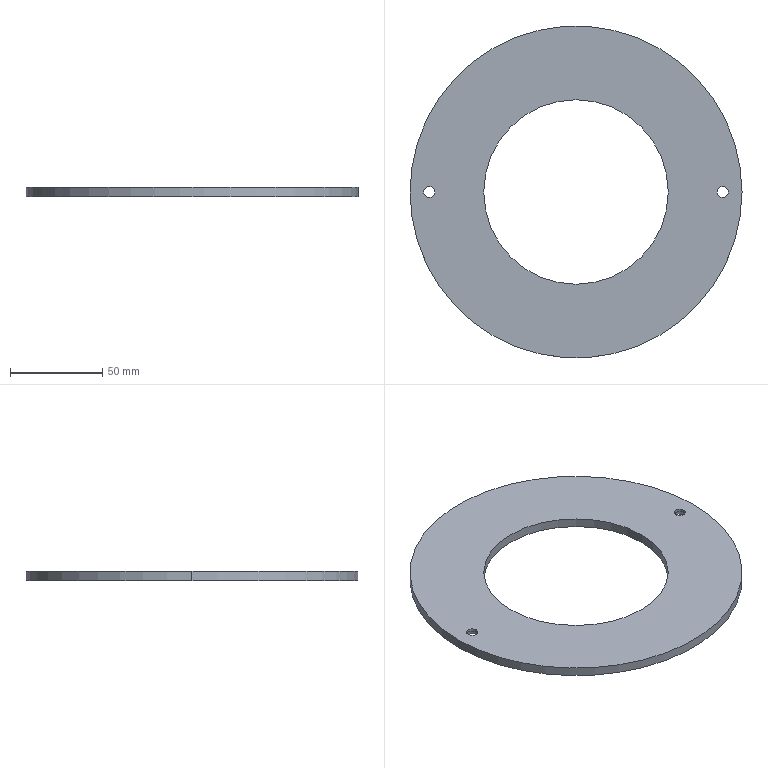Part | STEP file | Spacer block | 1 solid | 16 faces | box 180 x 180 x 5 mm | volume 87215 mm3 | cylinder 12 | plane 4 | commonest cylinder face diameters 6 x4 11 x4 100 x2 180 x2
STEP:
#1=CARTESIAN_POINT('',(85.05,0.,3.5));
#2=VERTEX_POINT('',#1);
#3=CARTESIAN_POINT('',(74.05,0.,3.5));
#4=VERTEX_POINT('',#3);
#5=CARTESIAN_POINT('',(79.55,0.,3.5));
#6=DIRECTION('',(0.,0.,-1.));
#7=DIRECTION('',(-1.,0.,0.));
#8=AXIS2_PLACEMENT_3D('',#5,#6,#7);
#9=CIRCLE('',#8,5.5);
#10=EDGE_CURVE('',#2,#4,#9,.T.);
#11=ORIENTED_EDGE('',*,*,#10,.F.);
#12=CARTESIAN_POINT('',(85.05,0.,0.));
#13=VERTEX_POINT('',#12);
#14=CARTESIAN_POINT('',(85.05,0.,3.5));
#15=DIRECTION('',(0.,0.,-1.));
#16=VECTOR('',#15,1000.);
#17=LINE('',#14,#16);
#18=EDGE_CURVE('',#2,#13,#17,.T.);
#19=ORIENTED_EDGE('',*,*,#18,.T.);
#20=CARTESIAN_POINT('',(74.05,0.,0.));
#21=VERTEX_POINT('',#20);
#22=CARTESIAN_POINT('',(79.55,0.,0.));
#23=DIRECTION('',(0.,0.,-1.));
#24=DIRECTION('',(-1.,0.,0.));
#25=AXIS2_PLACEMENT_3D('',#22,#23,#24);
#26=CIRCLE('',#25,5.5);
#27=EDGE_CURVE('',#13,#21,#26,.T.);
#28=ORIENTED_EDGE('',*,*,#27,.T.);
#29=CARTESIAN_POINT('',(74.05,0.,3.5));
#30=DIRECTION('',(0.,0.,-1.));
#31=VECTOR('',#30,1000.);
#32=LINE('',#29,#31);
#33=EDGE_CURVE('',#4,#21,#32,.T.);
#34=ORIENTED_EDGE('',*,*,#33,.F.);
#35=EDGE_LOOP('',(#11,#19,#28,#34));
#36=FACE_OUTER_BOUND('',#35,.T.);
#37=CARTESIAN_POINT('',(79.55,0.,3.5));
#38=DIRECTION('',(0.,0.,-1.));
#39=DIRECTION('',(-1.,0.,0.));
#40=AXIS2_PLACEMENT_3D('',#37,#38,#39);
#41=CYLINDRICAL_SURFACE('',#40,5.5);
#42=ADVANCED_FACE('',(#36),#41,.F.);
#43=CARTESIAN_POINT('',(-74.05,0.,3.5));
#44=VERTEX_POINT('',#43);
#45=CARTESIAN_POINT('',(-85.05,0.,3.5));
#46=VERTEX_POINT('',#45);
#47=CARTESIAN_POINT('',(-79.55,0.,3.5));
#48=DIRECTION('',(0.,0.,-1.));
#49=DIRECTION('',(-1.,0.,0.));
#50=AXIS2_PLACEMENT_3D('',#47,#48,#49);
#51=CIRCLE('',#50,5.5);
#52=EDGE_CURVE('',#44,#46,#51,.T.);
#53=ORIENTED_EDGE('',*,*,#52,.F.);
#54=CARTESIAN_POINT('',(-74.05,0.,0.));
#55=VERTEX_POINT('',#54);
#56=CARTESIAN_POINT('',(-74.05,0.,3.5));
#57=DIRECTION('',(0.,0.,-1.));
#58=VECTOR('',#57,1000.);
#59=LINE('',#56,#58);
#60=EDGE_CURVE('',#44,#55,#59,.T.);
#61=ORIENTED_EDGE('',*,*,#60,.T.);
#62=CARTESIAN_POINT('',(-85.05,0.,0.));
#63=VERTEX_POINT('',#62);
#64=CARTESIAN_POINT('',(-79.55,0.,0.));
#65=DIRECTION('',(0.,0.,-1.));
#66=DIRECTION('',(-1.,0.,0.));
#67=AXIS2_PLACEMENT_3D('',#64,#65,#66);
#68=CIRCLE('',#67,5.5);
#69=EDGE_CURVE('',#55,#63,#68,.T.);
#70=ORIENTED_EDGE('',*,*,#69,.T.);
#71=CARTESIAN_POINT('',(-85.05,0.,3.5));
#72=DIRECTION('',(0.,0.,-1.));
#73=VECTOR('',#72,1000.);
#74=LINE('',#71,#73);
#75=EDGE_CURVE('',#46,#63,#74,.T.);
#76=ORIENTED_EDGE('',*,*,#75,.F.);
#77=EDGE_LOOP('',(#53,#61,#70,#76));
#78=FACE_OUTER_BOUND('',#77,.T.);
#79=CARTESIAN_POINT('',(-79.55,0.,3.5));
#80=DIRECTION('',(0.,0.,-1.));
#81=DIRECTION('',(-1.,0.,0.));
#82=AXIS2_PLACEMENT_3D('',#79,#80,#81);
#83=CYLINDRICAL_SURFACE('',#82,5.5);
#84=ADVANCED_FACE('',(#78),#83,.F.);
#85=CARTESIAN_POINT('',(-50.,0.,5.));
#86=VERTEX_POINT('',#85);
#87=CARTESIAN_POINT('',(50.,0.,5.));
#88=VERTEX_POINT('',#87);
#89=CARTESIAN_POINT('',(0.,0.,5.));
#90=DIRECTION('',(0.,0.,1.));
#91=DIRECTION('',(1.,0.,0.));
#92=AXIS2_PLACEMENT_3D('',#89,#90,#91);
#93=CIRCLE('',#92,50.);
#94=EDGE_CURVE('',#86,#88,#93,.T.);
#95=ORIENTED_EDGE('',*,*,#94,.T.);
#96=CARTESIAN_POINT('',(50.,0.,0.));
#97=VERTEX_POINT('',#96);
#98=CARTESIAN_POINT('',(50.,0.,5.));
#99=DIRECTION('',(0.,0.,-1.));
#100=VECTOR('',#99,1000.);
#101=LINE('',#98,#100);
#102=EDGE_CURVE('',#88,#97,#101,.T.);
#103=ORIENTED_EDGE('',*,*,#102,.T.);
#104=CARTESIAN_POINT('',(-50.,0.,0.));
#105=VERTEX_POINT('',#104);
#106=CARTESIAN_POINT('',(0.,0.,0.));
#107=DIRECTION('',(0.,0.,1.));
#108=DIRECTION('',(1.,0.,0.));
#109=AXIS2_PLACEMENT_3D('',#106,#107,#108);
#110=CIRCLE('',#109,50.);
#111=EDGE_CURVE('',#105,#97,#110,.T.);
#112=ORIENTED_EDGE('',*,*,#111,.F.);
#113=CARTESIAN_POINT('',(-50.,0.,5.));
#114=DIRECTION('',(0.,0.,-1.));
#115=VECTOR('',#114,1000.);
#116=LINE('',#113,#115);
#117=EDGE_CURVE('',#86,#105,#116,.T.);
#118=ORIENTED_EDGE('',*,*,#117,.F.);
#119=EDGE_LOOP('',(#95,#103,#112,#118));
#120=FACE_OUTER_BOUND('',#119,.T.);
#121=CARTESIAN_POINT('',(0.,0.,5.));
#122=DIRECTION('',(0.,0.,-1.));
#123=DIRECTION('',(-1.,0.,0.));
#124=AXIS2_PLACEMENT_3D('',#121,#122,#123);
#125=CYLINDRICAL_SURFACE('',#124,50.);
#126=ADVANCED_FACE('',(#120),#125,.F.);
#127=CARTESIAN_POINT('',(90.,0.,5.));
#128=VERTEX_POINT('',#127);
#129=CARTESIAN_POINT('',(-90.,0.,5.));
#130=VERTEX_POINT('',#129);
#131=CARTESIAN_POINT('',(0.,0.,5.));
#132=DIRECTION('',(0.,0.,1.));
#133=DIRECTION('',(1.,0.,0.));
#134=AXIS2_PLACEMENT_3D('',#131,#132,#133);
#135=CIRCLE('',#134,90.);
#136=EDGE_CURVE('',#128,#130,#135,.T.);
#137=ORIENTED_EDGE('',*,*,#136,.F.);
#138=CARTESIAN_POINT('',(90.,0.,0.));
#139=VERTEX_POINT('',#138);
#140=CARTESIAN_POINT('',(90.,0.,5.));
#141=DIRECTION('',(0.,0.,-1.));
#142=VECTOR('',#141,1000.);
#143=LINE('',#140,#142);
#144=EDGE_CURVE('',#128,#139,#143,.T.);
#145=ORIENTED_EDGE('',*,*,#144,.T.);
#146=CARTESIAN_POINT('',(-90.,0.,0.));
#147=VERTEX_POINT('',#146);
#148=CARTESIAN_POINT('',(0.,0.,0.));
#149=DIRECTION('',(0.,0.,1.));
#150=DIRECTION('',(1.,0.,0.));
#151=AXIS2_PLACEMENT_3D('',#148,#149,#150);
#152=CIRCLE('',#151,90.);
#153=EDGE_CURVE('',#139,#147,#152,.T.);
#154=ORIENTED_EDGE('',*,*,#153,.T.);
#155=CARTESIAN_POINT('',(-90.,0.,5.));
#156=DIRECTION('',(0.,0.,-1.));
#157=VECTOR('',#156,1000.);
#158=LINE('',#155,#157);
#159=EDGE_CURVE('',#130,#147,#158,.T.);
#160=ORIENTED_EDGE('',*,*,#159,.F.);
#161=EDGE_LOOP('',(#137,#145,#154,#160));
#162=FACE_OUTER_BOUND('',#161,.T.);
#163=CARTESIAN_POINT('',(0.,0.,5.));
#164=DIRECTION('',(0.,0.,-1.));
#165=DIRECTION('',(-1.,0.,0.));
#166=AXIS2_PLACEMENT_3D('',#163,#164,#165);
#167=CYLINDRICAL_SURFACE('',#166,90.);
#168=ADVANCED_FACE('',(#162),#167,.T.);
#169=CARTESIAN_POINT('',(-82.55,0.,3.5));
#170=VERTEX_POINT('',#169);
#171=CARTESIAN_POINT('',(-76.55,0.,3.5));
#172=VERTEX_POINT('',#171);
#173=CARTESIAN_POINT('',(-79.55,0.,3.5));
#174=DIRECTION('',(0.,0.,1.));
#175=DIRECTION('',(-1.,0.,0.));
#176=AXIS2_PLACEMENT_3D('',#173,#174,#175);
#177=CIRCLE('',#176,3.);
#178=EDGE_CURVE('',#170,#172,#177,.T.);
#179=ORIENTED_EDGE('',*,*,#178,.F.);
#180=CARTESIAN_POINT('',(-82.55,0.,5.));
#181=VERTEX_POINT('',#180);
#182=CARTESIAN_POINT('',(-82.55,0.,-5.));
#183=DIRECTION('',(0.,0.,1.));
#184=VECTOR('',#183,1000.);
#185=LINE('',#182,#184);
#186=EDGE_CURVE('',#170,#181,#185,.T.);
#187=ORIENTED_EDGE('',*,*,#186,.T.);
#188=CARTESIAN_POINT('',(-76.55,0.,5.));
#189=VERTEX_POINT('',#188);
#190=CARTESIAN_POINT('',(-79.55,0.,5.));
#191=DIRECTION('',(0.,0.,1.));
#192=DIRECTION('',(1.,0.,0.));
#193=AXIS2_PLACEMENT_3D('',#190,#191,#192);
#194=CIRCLE('',#193,3.);
#195=EDGE_CURVE('',#181,#189,#194,.T.);
#196=ORIENTED_EDGE('',*,*,#195,.T.);
#197=CARTESIAN_POINT('',(-76.55,0.,-5.));
#198=DIRECTION('',(0.,0.,1.));
#199=VECTOR('',#198,1000.);
#200=LINE('',#197,#199);
#201=EDGE_CURVE('',#172,#189,#200,.T.);
#202=ORIENTED_EDGE('',*,*,#201,.F.);
#203=EDGE_LOOP('',(#179,#187,#196,#202));
#204=FACE_OUTER_BOUND('',#203,.T.);
#205=CARTESIAN_POINT('',(-79.55,0.,-5.));
#206=DIRECTION('',(0.,0.,1.));
#207=DIRECTION('',(1.,0.,0.));
#208=AXIS2_PLACEMENT_3D('',#205,#206,#207);
#209=CYLINDRICAL_SURFACE('',#208,3.);
#210=ADVANCED_FACE('',(#204),#209,.F.);
#211=CARTESIAN_POINT('',(76.55,0.,3.5));
#212=VERTEX_POINT('',#211);
#213=CARTESIAN_POINT('',(82.55,0.,3.5));
#214=VERTEX_POINT('',#213);
#215=CARTESIAN_POINT('',(79.55,0.,3.5));
#216=DIRECTION('',(0.,0.,1.));
#217=DIRECTION('',(-1.,0.,0.));
#218=AXIS2_PLACEMENT_3D('',#215,#216,#217);
#219=CIRCLE('',#218,3.);
#220=EDGE_CURVE('',#212,#214,#219,.T.);
#221=ORIENTED_EDGE('',*,*,#220,.F.);
#222=CARTESIAN_POINT('',(76.55,0.,5.));
#223=VERTEX_POINT('',#222);
#224=CARTESIAN_POINT('',(76.55,0.,-5.));
#225=DIRECTION('',(0.,0.,1.));
#226=VECTOR('',#225,1000.);
#227=LINE('',#224,#226);
#228=EDGE_CURVE('',#212,#223,#227,.T.);
#229=ORIENTED_EDGE('',*,*,#228,.T.);
#230=CARTESIAN_POINT('',(82.55,0.,5.));
#231=VERTEX_POINT('',#230);
#232=CARTESIAN_POINT('',(79.55,0.,5.));
#233=DIRECTION('',(0.,0.,1.));
#234=DIRECTION('',(1.,0.,0.));
#235=AXIS2_PLACEMENT_3D('',#232,#233,#234);
#236=CIRCLE('',#235,3.);
#237=EDGE_CURVE('',#223,#231,#236,.T.);
#238=ORIENTED_EDGE('',*,*,#237,.T.);
#239=CARTESIAN_POINT('',(82.55,0.,-5.));
#240=DIRECTION('',(0.,0.,1.));
#241=VECTOR('',#240,1000.);
#242=LINE('',#239,#241);
#243=EDGE_CURVE('',#214,#231,#242,.T.);
#244=ORIENTED_EDGE('',*,*,#243,.F.);
#245=EDGE_LOOP('',(#221,#229,#238,#244));
#246=FACE_OUTER_BOUND('',#245,.T.);
#247=CARTESIAN_POINT('',(79.55,0.,-5.));
#248=DIRECTION('',(0.,0.,1.));
#249=DIRECTION('',(1.,0.,0.));
#250=AXIS2_PLACEMENT_3D('',#247,#248,#249);
#251=CYLINDRICAL_SURFACE('',#250,3.);
#252=ADVANCED_FACE('',(#246),#251,.F.);
#253=ORIENTED_EDGE('',*,*,#228,.F.);
#254=CARTESIAN_POINT('',(79.55,0.,3.5));
#255=DIRECTION('',(0.,0.,1.));
#256=DIRECTION('',(-1.,0.,0.));
#257=AXIS2_PLACEMENT_3D('',#254,#255,#256);
#258=CIRCLE('',#257,3.);
#259=EDGE_CURVE('',#214,#212,#258,.T.);
#260=ORIENTED_EDGE('',*,*,#259,.F.);
#261=ORIENTED_EDGE('',*,*,#243,.T.);
#262=CARTESIAN_POINT('',(79.55,0.,5.));
#263=DIRECTION('',(0.,0.,1.));
#264=DIRECTION('',(1.,0.,0.));
#265=AXIS2_PLACEMENT_3D('',#262,#263,#264);
#266=CIRCLE('',#265,3.);
#267=EDGE_CURVE('',#231,#223,#266,.T.);
#268=ORIENTED_EDGE('',*,*,#267,.T.);
#269=EDGE_LOOP('',(#253,#260,#261,#268));
#270=FACE_OUTER_BOUND('',#269,.T.);
#271=CARTESIAN_POINT('',(79.55,0.,-5.));
#272=DIRECTION('',(0.,0.,1.));
#273=DIRECTION('',(1.,0.,0.));
#274=AXIS2_PLACEMENT_3D('',#271,#272,#273);
#275=CYLINDRICAL_SURFACE('',#274,3.);
#276=ADVANCED_FACE('',(#270),#275,.F.);
#277=ORIENTED_EDGE('',*,*,#186,.F.);
#278=CARTESIAN_POINT('',(-79.55,0.,3.5));
#279=DIRECTION('',(0.,0.,1.));
#280=DIRECTION('',(-1.,0.,0.));
#281=AXIS2_PLACEMENT_3D('',#278,#279,#280);
#282=CIRCLE('',#281,3.);
#283=EDGE_CURVE('',#172,#170,#282,.T.);
#284=ORIENTED_EDGE('',*,*,#283,.F.);
#285=ORIENTED_EDGE('',*,*,#201,.T.);
#286=CARTESIAN_POINT('',(-79.55,0.,5.));
#287=DIRECTION('',(0.,0.,1.));
#288=DIRECTION('',(1.,0.,0.));
#289=AXIS2_PLACEMENT_3D('',#286,#287,#288);
#290=CIRCLE('',#289,3.);
#291=EDGE_CURVE('',#189,#181,#290,.T.);
#292=ORIENTED_EDGE('',*,*,#291,.T.);
#293=EDGE_LOOP('',(#277,#284,#285,#292));
#294=FACE_OUTER_BOUND('',#293,.T.);
#295=CARTESIAN_POINT('',(-79.55,0.,-5.));
#296=DIRECTION('',(0.,0.,1.));
#297=DIRECTION('',(1.,0.,0.));
#298=AXIS2_PLACEMENT_3D('',#295,#296,#297);
#299=CYLINDRICAL_SURFACE('',#298,3.);
#300=ADVANCED_FACE('',(#294),#299,.F.);
#301=ORIENTED_EDGE('',*,*,#291,.F.);
#302=ORIENTED_EDGE('',*,*,#195,.F.);
#303=EDGE_LOOP('',(#301,#302));
#304=FACE_BOUND('',#303,.T.);
#305=ORIENTED_EDGE('',*,*,#267,.F.);
#306=ORIENTED_EDGE('',*,*,#237,.F.);
#307=EDGE_LOOP('',(#305,#306));
#308=FACE_BOUND('',#307,.T.);
#309=CARTESIAN_POINT('',(0.,0.,5.));
#310=DIRECTION('',(0.,0.,1.));
#311=DIRECTION('',(1.,0.,0.));
#312=AXIS2_PLACEMENT_3D('',#309,#310,#311);
#313=CIRCLE('',#312,90.);
#314=EDGE_CURVE('',#130,#128,#313,.T.);
#315=ORIENTED_EDGE('',*,*,#314,.T.);
#316=ORIENTED_EDGE('',*,*,#136,.T.);
#317=EDGE_LOOP('',(#315,#316));
#318=FACE_OUTER_BOUND('',#317,.T.);
#319=ORIENTED_EDGE('',*,*,#94,.F.);
#320=CARTESIAN_POINT('',(0.,0.,5.));
#321=DIRECTION('',(0.,0.,1.));
#322=DIRECTION('',(1.,0.,0.));
#323=AXIS2_PLACEMENT_3D('',#320,#321,#322);
#324=CIRCLE('',#323,50.);
#325=EDGE_CURVE('',#88,#86,#324,.T.);
#326=ORIENTED_EDGE('',*,*,#325,.F.);
#327=EDGE_LOOP('',(#319,#326));
#328=FACE_BOUND('',#327,.T.);
#329=CARTESIAN_POINT('',(0.,0.,5.));
#330=DIRECTION('',(0.,0.,1.));
#331=DIRECTION('',(1.,0.,0.));
#332=AXIS2_PLACEMENT_3D('',#329,#330,#331);
#333=PLANE('',#332);
#334=ADVANCED_FACE('',(#304,#308,#318,#328),#333,.T.);
#335=CARTESIAN_POINT('',(79.55,0.,0.));
#336=DIRECTION('',(0.,0.,-1.));
#337=DIRECTION('',(-1.,0.,0.));
#338=AXIS2_PLACEMENT_3D('',#335,#336,#337);
#339=CIRCLE('',#338,5.5);
#340=EDGE_CURVE('',#21,#13,#339,.T.);
#341=ORIENTED_EDGE('',*,*,#340,.F.);
#342=ORIENTED_EDGE('',*,*,#27,.F.);
#343=EDGE_LOOP('',(#341,#342));
#344=FACE_BOUND('',#343,.T.);
#345=CARTESIAN_POINT('',(-79.55,0.,0.));
#346=DIRECTION('',(0.,0.,-1.));
#347=DIRECTION('',(-1.,0.,0.));
#348=AXIS2_PLACEMENT_3D('',#345,#346,#347);
#349=CIRCLE('',#348,5.5);
#350=EDGE_CURVE('',#63,#55,#349,.T.);
#351=ORIENTED_EDGE('',*,*,#350,.F.);
#352=ORIENTED_EDGE('',*,*,#69,.F.);
#353=EDGE_LOOP('',(#351,#352));
#354=FACE_BOUND('',#353,.T.);
#355=CARTESIAN_POINT('',(0.,0.,0.));
#356=DIRECTION('',(0.,0.,1.));
#357=DIRECTION('',(1.,0.,0.));
#358=AXIS2_PLACEMENT_3D('',#355,#356,#357);
#359=CIRCLE('',#358,90.);
#360=EDGE_CURVE('',#147,#139,#359,.T.);
#361=ORIENTED_EDGE('',*,*,#360,.F.);
#362=ORIENTED_EDGE('',*,*,#153,.F.);
#363=EDGE_LOOP('',(#361,#362));
#364=FACE_OUTER_BOUND('',#363,.T.);
#365=ORIENTED_EDGE('',*,*,#111,.T.);
#366=CARTESIAN_POINT('',(0.,0.,0.));
#367=DIRECTION('',(0.,0.,1.));
#368=DIRECTION('',(1.,0.,0.));
#369=AXIS2_PLACEMENT_3D('',#366,#367,#368);
#370=CIRCLE('',#369,50.);
#371=EDGE_CURVE('',#97,#105,#370,.T.);
#372=ORIENTED_EDGE('',*,*,#371,.T.);
#373=EDGE_LOOP('',(#365,#372));
#374=FACE_BOUND('',#373,.T.);
#375=CARTESIAN_POINT('',(0.,0.,0.));
#376=DIRECTION('',(0.,0.,1.));
#377=DIRECTION('',(1.,0.,0.));
#378=AXIS2_PLACEMENT_3D('',#375,#376,#377);
#379=PLANE('',#378);
#380=ADVANCED_FACE('',(#344,#354,#364,#374),#379,.F.);
#381=ORIENTED_EDGE('',*,*,#144,.F.);
#382=ORIENTED_EDGE('',*,*,#314,.F.);
#383=ORIENTED_EDGE('',*,*,#159,.T.);
#384=ORIENTED_EDGE('',*,*,#360,.T.);
#385=EDGE_LOOP('',(#381,#382,#383,#384));
#386=FACE_OUTER_BOUND('',#385,.T.);
#387=CARTESIAN_POINT('',(0.,0.,5.));
#388=DIRECTION('',(0.,0.,-1.));
#389=DIRECTION('',(-1.,0.,0.));
#390=AXIS2_PLACEMENT_3D('',#387,#388,#389);
#391=CYLINDRICAL_SURFACE('',#390,90.);
#392=ADVANCED_FACE('',(#386),#391,.T.);
#393=ORIENTED_EDGE('',*,*,#102,.F.);
#394=ORIENTED_EDGE('',*,*,#325,.T.);
#395=ORIENTED_EDGE('',*,*,#117,.T.);
#396=ORIENTED_EDGE('',*,*,#371,.F.);
#397=EDGE_LOOP('',(#393,#394,#395,#396));
#398=FACE_OUTER_BOUND('',#397,.T.);
#399=CARTESIAN_POINT('',(0.,0.,5.));
#400=DIRECTION('',(0.,0.,-1.));
#401=DIRECTION('',(-1.,0.,0.));
#402=AXIS2_PLACEMENT_3D('',#399,#400,#401);
#403=CYLINDRICAL_SURFACE('',#402,50.);
#404=ADVANCED_FACE('',(#398),#403,.F.);
#405=CARTESIAN_POINT('',(-79.55,0.,3.5));
#406=DIRECTION('',(0.,0.,-1.));
#407=DIRECTION('',(-1.,0.,0.));
#408=AXIS2_PLACEMENT_3D('',#405,#406,#407);
#409=CIRCLE('',#408,5.5);
#410=EDGE_CURVE('',#46,#44,#409,.T.);
#411=ORIENTED_EDGE('',*,*,#410,.T.);
#412=ORIENTED_EDGE('',*,*,#52,.T.);
#413=EDGE_LOOP('',(#411,#412));
#414=FACE_OUTER_BOUND('',#413,.T.);
#415=ORIENTED_EDGE('',*,*,#283,.T.);
#416=ORIENTED_EDGE('',*,*,#178,.T.);
#417=EDGE_LOOP('',(#415,#416));
#418=FACE_BOUND('',#417,.T.);
#419=CARTESIAN_POINT('',(-79.55,0.,3.5));
#420=DIRECTION('',(0.,0.,-1.));
#421=DIRECTION('',(-1.,0.,0.));
#422=AXIS2_PLACEMENT_3D('',#419,#420,#421);
#423=PLANE('',#422);
#424=ADVANCED_FACE('',(#414,#418),#423,.T.);
#425=ORIENTED_EDGE('',*,*,#60,.F.);
#426=ORIENTED_EDGE('',*,*,#410,.F.);
#427=ORIENTED_EDGE('',*,*,#75,.T.);
#428=ORIENTED_EDGE('',*,*,#350,.T.);
#429=EDGE_LOOP('',(#425,#426,#427,#428));
#430=FACE_OUTER_BOUND('',#429,.T.);
#431=CARTESIAN_POINT('',(-79.55,0.,3.5));
#432=DIRECTION('',(0.,0.,-1.));
#433=DIRECTION('',(-1.,0.,0.));
#434=AXIS2_PLACEMENT_3D('',#431,#432,#433);
#435=CYLINDRICAL_SURFACE('',#434,5.5);
#436=ADVANCED_FACE('',(#430),#435,.F.);
#437=CARTESIAN_POINT('',(79.55,0.,3.5));
#438=DIRECTION('',(0.,0.,-1.));
#439=DIRECTION('',(-1.,0.,0.));
#440=AXIS2_PLACEMENT_3D('',#437,#438,#439);
#441=CIRCLE('',#440,5.5);
#442=EDGE_CURVE('',#4,#2,#441,.T.);
#443=ORIENTED_EDGE('',*,*,#442,.T.);
#444=ORIENTED_EDGE('',*,*,#10,.T.);
#445=EDGE_LOOP('',(#443,#444));
#446=FACE_OUTER_BOUND('',#445,.T.);
#447=ORIENTED_EDGE('',*,*,#259,.T.);
#448=ORIENTED_EDGE('',*,*,#220,.T.);
#449=EDGE_LOOP('',(#447,#448));
#450=FACE_BOUND('',#449,.T.);
#451=CARTESIAN_POINT('',(79.55,0.,3.5));
#452=DIRECTION('',(0.,0.,-1.));
#453=DIRECTION('',(-1.,0.,0.));
#454=AXIS2_PLACEMENT_3D('',#451,#452,#453);
#455=PLANE('',#454);
#456=ADVANCED_FACE('',(#446,#450),#455,.T.);
#457=ORIENTED_EDGE('',*,*,#18,.F.);
#458=ORIENTED_EDGE('',*,*,#442,.F.);
#459=ORIENTED_EDGE('',*,*,#33,.T.);
#460=ORIENTED_EDGE('',*,*,#340,.T.);
#461=EDGE_LOOP('',(#457,#458,#459,#460));
#462=FACE_OUTER_BOUND('',#461,.T.);
#463=CARTESIAN_POINT('',(79.55,0.,3.5));
#464=DIRECTION('',(0.,0.,-1.));
#465=DIRECTION('',(-1.,0.,0.));
#466=AXIS2_PLACEMENT_3D('',#463,#464,#465);
#467=CYLINDRICAL_SURFACE('',#466,5.5);
#468=ADVANCED_FACE('',(#462),#467,.F.);
#469=CLOSED_SHELL('',(#42,#84,#126,#168,#210,#252,#276,#300,#334,#380,#392,#404,#424,#436,#456,#468));
#470=MANIFOLD_SOLID_BREP('',#469);
#471=CARTESIAN_POINT('',(0.,0.,0.));
#472=DIRECTION('',(0.,0.,1.));
#473=DIRECTION('',(1.,0.,0.));
#474=AXIS2_PLACEMENT_3D('',#471,#472,#473);
#475=(LENGTH_UNIT()NAMED_UNIT(*)SI_UNIT(.MILLI.,.METRE.));
#476=UNCERTAINTY_MEASURE_WITH_UNIT(LENGTH_MEASURE(0.00001),#475,'','');
#477=(NAMED_UNIT(*)PLANE_ANGLE_UNIT()SI_UNIT($,.RADIAN.));
#478=(NAMED_UNIT(*)SI_UNIT($,.STERADIAN.)SOLID_ANGLE_UNIT());
#479=(GEOMETRIC_REPRESENTATION_CONTEXT(3)GLOBAL_UNCERTAINTY_ASSIGNED_CONTEXT((#476))GLOBAL_UNIT_ASSIGNED_CONTEXT((#475,#477,#478))REPRESENTATION_CONTEXT('',''));
#480=ADVANCED_BREP_SHAPE_REPRESENTATION('',(#470,#474),#479);